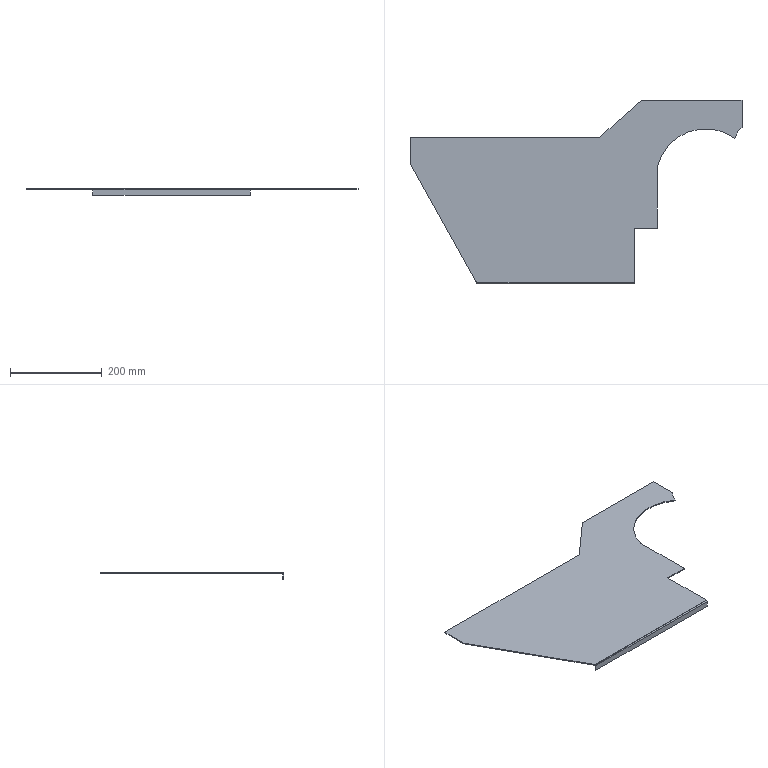Part | STEP file | TX-003-1 | 1 solid | 21 faces | box 722 x 399 x 15 mm | volume 342555 mm3 | plane 16 | cylinder 5 | commonest cylinder face diameters 1 x2 5 x1 78.426 x1 216 x1
STEP:
#1=CARTESIAN_POINT('',(-209.508,-144.397,0.));
#2=VERTEX_POINT('',#1);
#3=CARTESIAN_POINT('',(-209.508,-143.397,0.));
#4=VERTEX_POINT('',#3);
#5=CARTESIAN_POINT('',(-209.508,-143.397,0.));
#6=DIRECTION('',(0.,1.,0.));
#7=VECTOR('',#6,1000.);
#8=LINE('',#5,#7);
#9=EDGE_CURVE('',#2,#4,#8,.T.);
#10=ORIENTED_EDGE('',*,*,#9,.F.);
#11=CARTESIAN_POINT('',(132.378,-144.397,0.));
#12=VERTEX_POINT('',#11);
#13=CARTESIAN_POINT('',(287.878,-144.397,0.));
#14=DIRECTION('',(1.,0.,0.));
#15=VECTOR('',#14,1000.);
#16=LINE('',#13,#15);
#17=EDGE_CURVE('',#2,#12,#16,.T.);
#18=ORIENTED_EDGE('',*,*,#17,.T.);
#19=CARTESIAN_POINT('',(132.378,-25.897,0.));
#20=VERTEX_POINT('',#19);
#21=CARTESIAN_POINT('',(132.378,82.103,0.));
#22=DIRECTION('',(0.,1.,0.));
#23=VECTOR('',#22,1000.);
#24=LINE('',#21,#23);
#25=EDGE_CURVE('',#12,#20,#24,.T.);
#26=ORIENTED_EDGE('',*,*,#25,.T.);
#27=CARTESIAN_POINT('',(182.878,-25.897,0.));
#28=VERTEX_POINT('',#27);
#29=CARTESIAN_POINT('',(287.878,-25.897,0.));
#30=DIRECTION('',(1.,0.,0.));
#31=VECTOR('',#30,1000.);
#32=LINE('',#29,#31);
#33=EDGE_CURVE('',#20,#28,#32,.T.);
#34=ORIENTED_EDGE('',*,*,#33,.T.);
#35=CARTESIAN_POINT('',(182.878,107.381,0.));
#36=VERTEX_POINT('',#35);
#37=CARTESIAN_POINT('',(182.878,82.103,0.));
#38=DIRECTION('',(0.,1.,0.));
#39=VECTOR('',#38,1000.);
#40=LINE('',#37,#39);
#41=EDGE_CURVE('',#28,#36,#40,.T.);
#42=ORIENTED_EDGE('',*,*,#41,.T.);
#43=CARTESIAN_POINT('',(351.619,169.287,0.));
#44=VERTEX_POINT('',#43);
#45=CARTESIAN_POINT('',(287.878,82.103,0.));
#46=DIRECTION('',(0.,0.,-1.));
#47=DIRECTION('',(1.,0.,0.));
#48=AXIS2_PLACEMENT_3D('',#45,#46,#47);
#49=CIRCLE('',#48,108.);
#50=EDGE_CURVE('',#36,#44,#49,.T.);
#51=ORIENTED_EDGE('',*,*,#50,.T.);
#52=CARTESIAN_POINT('',(366.878,193.103,0.));
#53=VERTEX_POINT('',#52);
#54=CARTESIAN_POINT('',(390.044,161.464,0.));
#55=DIRECTION('',(0.,0.,-1.));
#56=DIRECTION('',(1.,0.,0.));
#57=AXIS2_PLACEMENT_3D('',#54,#55,#56);
#58=CIRCLE('',#57,39.213);
#59=EDGE_CURVE('',#44,#53,#58,.T.);
#60=ORIENTED_EDGE('',*,*,#59,.T.);
#61=CARTESIAN_POINT('',(366.878,252.103,0.));
#62=VERTEX_POINT('',#61);
#63=CARTESIAN_POINT('',(366.878,82.103,0.));
#64=DIRECTION('',(0.,1.,0.));
#65=VECTOR('',#64,1000.);
#66=LINE('',#63,#65);
#67=EDGE_CURVE('',#53,#62,#66,.T.);
#68=ORIENTED_EDGE('',*,*,#67,.T.);
#69=CARTESIAN_POINT('',(147.878,252.103,0.));
#70=VERTEX_POINT('',#69);
#71=CARTESIAN_POINT('',(287.878,252.103,0.));
#72=DIRECTION('',(-1.,0.,0.));
#73=VECTOR('',#72,1000.);
#74=LINE('',#71,#73);
#75=EDGE_CURVE('',#62,#70,#74,.T.);
#76=ORIENTED_EDGE('',*,*,#75,.T.);
#77=CARTESIAN_POINT('',(57.878,172.103,0.));
#78=VERTEX_POINT('',#77);
#79=CARTESIAN_POINT('',(147.878,252.103,0.));
#80=DIRECTION('',(-0.7474,-0.6644,0.));
#81=VECTOR('',#80,1000.);
#82=LINE('',#79,#81);
#83=EDGE_CURVE('',#70,#78,#82,.T.);
#84=ORIENTED_EDGE('',*,*,#83,.T.);
#85=CARTESIAN_POINT('',(-355.122,172.103,0.));
#86=VERTEX_POINT('',#85);
#87=CARTESIAN_POINT('',(287.878,172.103,0.));
#88=DIRECTION('',(-1.,0.,0.));
#89=VECTOR('',#88,1000.);
#90=LINE('',#87,#89);
#91=EDGE_CURVE('',#78,#86,#90,.T.);
#92=ORIENTED_EDGE('',*,*,#91,.T.);
#93=CARTESIAN_POINT('',(-355.122,114.103,0.));
#94=VERTEX_POINT('',#93);
#95=CARTESIAN_POINT('',(-355.122,82.103,0.));
#96=DIRECTION('',(0.,-1.,0.));
#97=VECTOR('',#96,1000.);
#98=LINE('',#95,#97);
#99=EDGE_CURVE('',#86,#94,#98,.T.);
#100=ORIENTED_EDGE('',*,*,#99,.T.);
#101=CARTESIAN_POINT('',(-210.508,-145.105,0.));
#102=VERTEX_POINT('',#101);
#103=CARTESIAN_POINT('',(-355.122,114.103,0.));
#104=DIRECTION('',(0.4872,-0.8733,0.));
#105=VECTOR('',#104,1000.);
#106=LINE('',#103,#105);
#107=EDGE_CURVE('',#94,#102,#106,.T.);
#108=ORIENTED_EDGE('',*,*,#107,.T.);
#109=CARTESIAN_POINT('',(-210.508,-143.397,0.));
#110=VERTEX_POINT('',#109);
#111=CARTESIAN_POINT('',(-210.508,-145.105,0.));
#112=DIRECTION('',(0.,-1.,0.));
#113=VECTOR('',#112,1000.);
#114=LINE('',#111,#113);
#115=EDGE_CURVE('',#110,#102,#114,.T.);
#116=ORIENTED_EDGE('',*,*,#115,.F.);
#117=CARTESIAN_POINT('',(-210.008,-143.397,0.));
#118=DIRECTION('',(0.,0.,-1.));
#119=DIRECTION('',(1.,0.,0.));
#120=AXIS2_PLACEMENT_3D('',#117,#118,#119);
#121=CIRCLE('',#120,0.5);
#122=EDGE_CURVE('',#110,#4,#121,.T.);
#123=ORIENTED_EDGE('',*,*,#122,.T.);
#124=EDGE_LOOP('',(#10,#18,#26,#34,#42,#51,#60,#68,#76,#84,#92,#100,#108,#116,#123));
#125=FACE_OUTER_BOUND('',#124,.T.);
#126=CARTESIAN_POINT('',(287.878,82.103,0.));
#127=DIRECTION('',(0.,0.,1.));
#128=DIRECTION('',(1.,0.,0.));
#129=AXIS2_PLACEMENT_3D('',#126,#127,#128);
#130=PLANE('',#129);
#131=ADVANCED_FACE('',(#125),#130,.T.);
#132=CARTESIAN_POINT('',(-209.508,-146.897,-2.5));
#133=VERTEX_POINT('',#132);
#134=CARTESIAN_POINT('',(-209.508,-144.397,-2.5));
#135=DIRECTION('',(1.,0.,0.));
#136=DIRECTION('',(0.,0.,1.));
#137=AXIS2_PLACEMENT_3D('',#134,#135,#136);
#138=CIRCLE('',#137,2.5);
#139=EDGE_CURVE('',#2,#133,#138,.T.);
#140=ORIENTED_EDGE('',*,*,#139,.T.);
#141=CARTESIAN_POINT('',(132.378,-146.897,-2.5));
#142=VERTEX_POINT('',#141);
#143=CARTESIAN_POINT('',(-209.508,-146.897,-2.5));
#144=DIRECTION('',(1.,0.,0.));
#145=VECTOR('',#144,1000.);
#146=LINE('',#143,#145);
#147=EDGE_CURVE('',#133,#142,#146,.T.);
#148=ORIENTED_EDGE('',*,*,#147,.T.);
#149=CARTESIAN_POINT('',(132.378,-144.397,-2.5));
#150=DIRECTION('',(-1.,0.,0.));
#151=DIRECTION('',(0.,0.,1.));
#152=AXIS2_PLACEMENT_3D('',#149,#150,#151);
#153=CIRCLE('',#152,2.5);
#154=EDGE_CURVE('',#142,#12,#153,.T.);
#155=ORIENTED_EDGE('',*,*,#154,.T.);
#156=ORIENTED_EDGE('',*,*,#17,.F.);
#157=EDGE_LOOP('',(#140,#148,#155,#156));
#158=FACE_OUTER_BOUND('',#157,.T.);
#159=CARTESIAN_POINT('',(-209.508,-144.397,-2.5));
#160=DIRECTION('',(-1.,0.,0.));
#161=DIRECTION('',(0.,0.,1.));
#162=AXIS2_PLACEMENT_3D('',#159,#160,#161);
#163=CYLINDRICAL_SURFACE('',#162,2.5);
#164=ADVANCED_FACE('',(#158),#163,.T.);
#165=ORIENTED_EDGE('',*,*,#107,.F.);
#166=CARTESIAN_POINT('',(-355.122,114.103,-2.));
#167=VERTEX_POINT('',#166);
#168=CARTESIAN_POINT('',(-355.122,114.103,-2.));
#169=DIRECTION('',(0.,0.,-1.));
#170=VECTOR('',#169,1000.);
#171=LINE('',#168,#170);
#172=EDGE_CURVE('',#94,#167,#171,.T.);
#173=ORIENTED_EDGE('',*,*,#172,.T.);
#174=CARTESIAN_POINT('',(-210.508,-145.105,-2.));
#175=VERTEX_POINT('',#174);
#176=CARTESIAN_POINT('',(-355.122,114.103,-2.));
#177=DIRECTION('',(0.4872,-0.8733,0.));
#178=VECTOR('',#177,1000.);
#179=LINE('',#176,#178);
#180=EDGE_CURVE('',#167,#175,#179,.T.);
#181=ORIENTED_EDGE('',*,*,#180,.T.);
#182=CARTESIAN_POINT('',(-210.508,-145.105,-2.));
#183=DIRECTION('',(0.,0.,1.));
#184=VECTOR('',#183,1000.);
#185=LINE('',#182,#184);
#186=EDGE_CURVE('',#175,#102,#185,.T.);
#187=ORIENTED_EDGE('',*,*,#186,.T.);
#188=EDGE_LOOP('',(#165,#173,#181,#187));
#189=FACE_OUTER_BOUND('',#188,.T.);
#190=CARTESIAN_POINT('',(-355.122,114.103,-2.));
#191=DIRECTION('',(-0.8733,-0.4872,0.));
#192=DIRECTION('',(0.4872,-0.8733,0.));
#193=AXIS2_PLACEMENT_3D('',#190,#191,#192);
#194=PLANE('',#193);
#195=ADVANCED_FACE('',(#189),#194,.T.);
#196=CARTESIAN_POINT('',(-355.122,172.103,-2.));
#197=VERTEX_POINT('',#196);
#198=CARTESIAN_POINT('',(-355.122,114.103,-2.));
#199=DIRECTION('',(0.,-1.,0.));
#200=VECTOR('',#199,1000.);
#201=LINE('',#198,#200);
#202=EDGE_CURVE('',#197,#167,#201,.T.);
#203=ORIENTED_EDGE('',*,*,#202,.T.);
#204=ORIENTED_EDGE('',*,*,#172,.F.);
#205=ORIENTED_EDGE('',*,*,#99,.F.);
#206=CARTESIAN_POINT('',(-355.122,172.103,-2.));
#207=DIRECTION('',(0.,0.,-1.));
#208=VECTOR('',#207,1000.);
#209=LINE('',#206,#208);
#210=EDGE_CURVE('',#86,#197,#209,.T.);
#211=ORIENTED_EDGE('',*,*,#210,.T.);
#212=EDGE_LOOP('',(#203,#204,#205,#211));
#213=FACE_OUTER_BOUND('',#212,.T.);
#214=CARTESIAN_POINT('',(-355.122,114.103,-2.));
#215=DIRECTION('',(-1.,0.,0.));
#216=DIRECTION('',(0.,-1.,0.));
#217=AXIS2_PLACEMENT_3D('',#214,#215,#216);
#218=PLANE('',#217);
#219=ADVANCED_FACE('',(#213),#218,.T.);
#220=CARTESIAN_POINT('',(57.878,172.103,-2.));
#221=VERTEX_POINT('',#220);
#222=CARTESIAN_POINT('',(-355.122,172.103,-2.));
#223=DIRECTION('',(-1.,0.,0.));
#224=VECTOR('',#223,1000.);
#225=LINE('',#222,#224);
#226=EDGE_CURVE('',#221,#197,#225,.T.);
#227=ORIENTED_EDGE('',*,*,#226,.T.);
#228=ORIENTED_EDGE('',*,*,#210,.F.);
#229=ORIENTED_EDGE('',*,*,#91,.F.);
#230=CARTESIAN_POINT('',(57.878,172.103,-2.));
#231=DIRECTION('',(0.,0.,-1.));
#232=VECTOR('',#231,1000.);
#233=LINE('',#230,#232);
#234=EDGE_CURVE('',#78,#221,#233,.T.);
#235=ORIENTED_EDGE('',*,*,#234,.T.);
#236=EDGE_LOOP('',(#227,#228,#229,#235));
#237=FACE_OUTER_BOUND('',#236,.T.);
#238=CARTESIAN_POINT('',(-355.122,172.103,-2.));
#239=DIRECTION('',(0.,1.,0.));
#240=DIRECTION('',(-1.,0.,0.));
#241=AXIS2_PLACEMENT_3D('',#238,#239,#240);
#242=PLANE('',#241);
#243=ADVANCED_FACE('',(#237),#242,.T.);
#244=CARTESIAN_POINT('',(147.878,252.103,-2.));
#245=VERTEX_POINT('',#244);
#246=CARTESIAN_POINT('',(57.878,172.103,-2.));
#247=DIRECTION('',(-0.7474,-0.6644,0.));
#248=VECTOR('',#247,1000.);
#249=LINE('',#246,#248);
#250=EDGE_CURVE('',#245,#221,#249,.T.);
#251=ORIENTED_EDGE('',*,*,#250,.T.);
#252=ORIENTED_EDGE('',*,*,#234,.F.);
#253=ORIENTED_EDGE('',*,*,#83,.F.);
#254=CARTESIAN_POINT('',(147.878,252.103,-2.));
#255=DIRECTION('',(0.,0.,-1.));
#256=VECTOR('',#255,1000.);
#257=LINE('',#254,#256);
#258=EDGE_CURVE('',#70,#245,#257,.T.);
#259=ORIENTED_EDGE('',*,*,#258,.T.);
#260=EDGE_LOOP('',(#251,#252,#253,#259));
#261=FACE_OUTER_BOUND('',#260,.T.);
#262=CARTESIAN_POINT('',(57.878,172.103,-2.));
#263=DIRECTION('',(-0.6644,0.7474,0.));
#264=DIRECTION('',(-0.7474,-0.6644,0.));
#265=AXIS2_PLACEMENT_3D('',#262,#263,#264);
#266=PLANE('',#265);
#267=ADVANCED_FACE('',(#261),#266,.T.);
#268=CARTESIAN_POINT('',(366.878,252.103,-2.));
#269=VERTEX_POINT('',#268);
#270=CARTESIAN_POINT('',(147.878,252.103,-2.));
#271=DIRECTION('',(-1.,0.,0.));
#272=VECTOR('',#271,1000.);
#273=LINE('',#270,#272);
#274=EDGE_CURVE('',#269,#245,#273,.T.);
#275=ORIENTED_EDGE('',*,*,#274,.T.);
#276=ORIENTED_EDGE('',*,*,#258,.F.);
#277=ORIENTED_EDGE('',*,*,#75,.F.);
#278=CARTESIAN_POINT('',(366.878,252.103,-2.));
#279=DIRECTION('',(0.,0.,-1.));
#280=VECTOR('',#279,1000.);
#281=LINE('',#278,#280);
#282=EDGE_CURVE('',#62,#269,#281,.T.);
#283=ORIENTED_EDGE('',*,*,#282,.T.);
#284=EDGE_LOOP('',(#275,#276,#277,#283));
#285=FACE_OUTER_BOUND('',#284,.T.);
#286=CARTESIAN_POINT('',(147.878,252.103,-2.));
#287=DIRECTION('',(0.,1.,0.));
#288=DIRECTION('',(-1.,0.,0.));
#289=AXIS2_PLACEMENT_3D('',#286,#287,#288);
#290=PLANE('',#289);
#291=ADVANCED_FACE('',(#285),#290,.T.);
#292=CARTESIAN_POINT('',(366.878,193.103,-2.));
#293=VERTEX_POINT('',#292);
#294=CARTESIAN_POINT('',(366.878,193.103,-2.));
#295=DIRECTION('',(0.,1.,0.));
#296=VECTOR('',#295,1000.);
#297=LINE('',#294,#296);
#298=EDGE_CURVE('',#293,#269,#297,.T.);
#299=ORIENTED_EDGE('',*,*,#298,.T.);
#300=ORIENTED_EDGE('',*,*,#282,.F.);
#301=ORIENTED_EDGE('',*,*,#67,.F.);
#302=CARTESIAN_POINT('',(366.878,193.103,-2.));
#303=DIRECTION('',(0.,0.,-1.));
#304=VECTOR('',#303,1000.);
#305=LINE('',#302,#304);
#306=EDGE_CURVE('',#53,#293,#305,.T.);
#307=ORIENTED_EDGE('',*,*,#306,.T.);
#308=EDGE_LOOP('',(#299,#300,#301,#307));
#309=FACE_OUTER_BOUND('',#308,.T.);
#310=CARTESIAN_POINT('',(366.878,193.103,-2.));
#311=DIRECTION('',(1.,0.,0.));
#312=DIRECTION('',(0.,0.,-1.));
#313=AXIS2_PLACEMENT_3D('',#310,#311,#312);
#314=PLANE('',#313);
#315=ADVANCED_FACE('',(#309),#314,.T.);
#316=CARTESIAN_POINT('',(351.619,169.287,-2.));
#317=VERTEX_POINT('',#316);
#318=CARTESIAN_POINT('',(351.619,169.287,-2.));
#319=DIRECTION('',(0.,0.,1.));
#320=VECTOR('',#319,1000.);
#321=LINE('',#318,#320);
#322=EDGE_CURVE('',#317,#44,#321,.T.);
#323=ORIENTED_EDGE('',*,*,#322,.F.);
#324=CARTESIAN_POINT('',(390.044,161.464,-2.));
#325=DIRECTION('',(0.,0.,1.));
#326=DIRECTION('',(1.,0.,0.));
#327=AXIS2_PLACEMENT_3D('',#324,#325,#326);
#328=CIRCLE('',#327,39.213);
#329=EDGE_CURVE('',#293,#317,#328,.T.);
#330=ORIENTED_EDGE('',*,*,#329,.F.);
#331=ORIENTED_EDGE('',*,*,#306,.F.);
#332=ORIENTED_EDGE('',*,*,#59,.F.);
#333=EDGE_LOOP('',(#323,#330,#331,#332));
#334=FACE_OUTER_BOUND('',#333,.T.);
#335=CARTESIAN_POINT('',(390.044,161.464,-2.));
#336=DIRECTION('',(0.,0.,1.));
#337=DIRECTION('',(1.,0.,0.));
#338=AXIS2_PLACEMENT_3D('',#335,#336,#337);
#339=CYLINDRICAL_SURFACE('',#338,39.213);
#340=ADVANCED_FACE('',(#334),#339,.F.);
#341=CARTESIAN_POINT('',(182.878,107.381,-2.));
#342=VERTEX_POINT('',#341);
#343=CARTESIAN_POINT('',(182.878,107.381,-2.));
#344=DIRECTION('',(0.,0.,1.));
#345=VECTOR('',#344,1000.);
#346=LINE('',#343,#345);
#347=EDGE_CURVE('',#342,#36,#346,.T.);
#348=ORIENTED_EDGE('',*,*,#347,.F.);
#349=CARTESIAN_POINT('',(287.878,82.103,-2.));
#350=DIRECTION('',(0.,0.,1.));
#351=DIRECTION('',(1.,0.,0.));
#352=AXIS2_PLACEMENT_3D('',#349,#350,#351);
#353=CIRCLE('',#352,108.);
#354=EDGE_CURVE('',#317,#342,#353,.T.);
#355=ORIENTED_EDGE('',*,*,#354,.F.);
#356=ORIENTED_EDGE('',*,*,#322,.T.);
#357=ORIENTED_EDGE('',*,*,#50,.F.);
#358=EDGE_LOOP('',(#348,#355,#356,#357));
#359=FACE_OUTER_BOUND('',#358,.T.);
#360=CARTESIAN_POINT('',(287.878,82.103,-2.));
#361=DIRECTION('',(0.,0.,1.));
#362=DIRECTION('',(1.,0.,0.));
#363=AXIS2_PLACEMENT_3D('',#360,#361,#362);
#364=CYLINDRICAL_SURFACE('',#363,108.);
#365=ADVANCED_FACE('',(#359),#364,.F.);
#366=ORIENTED_EDGE('',*,*,#347,.T.);
#367=ORIENTED_EDGE('',*,*,#41,.F.);
#368=CARTESIAN_POINT('',(182.878,-25.897,-2.));
#369=VERTEX_POINT('',#368);
#370=CARTESIAN_POINT('',(182.878,-25.897,-2.));
#371=DIRECTION('',(0.,0.,-1.));
#372=VECTOR('',#371,1000.);
#373=LINE('',#370,#372);
#374=EDGE_CURVE('',#28,#369,#373,.T.);
#375=ORIENTED_EDGE('',*,*,#374,.T.);
#376=CARTESIAN_POINT('',(182.878,107.381,-2.));
#377=DIRECTION('',(0.,1.,0.));
#378=VECTOR('',#377,1000.);
#379=LINE('',#376,#378);
#380=EDGE_CURVE('',#369,#342,#379,.T.);
#381=ORIENTED_EDGE('',*,*,#380,.T.);
#382=EDGE_LOOP('',(#366,#367,#375,#381));
#383=FACE_OUTER_BOUND('',#382,.T.);
#384=CARTESIAN_POINT('',(182.878,107.381,-2.));
#385=DIRECTION('',(1.,0.,0.));
#386=DIRECTION('',(0.,1.,0.));
#387=AXIS2_PLACEMENT_3D('',#384,#385,#386);
#388=PLANE('',#387);
#389=ADVANCED_FACE('',(#383),#388,.T.);
#390=ORIENTED_EDGE('',*,*,#33,.F.);
#391=CARTESIAN_POINT('',(132.378,-25.897,-2.));
#392=VERTEX_POINT('',#391);
#393=CARTESIAN_POINT('',(132.378,-25.897,-15.));
#394=DIRECTION('',(0.,0.,1.));
#395=VECTOR('',#394,1000.);
#396=LINE('',#393,#395);
#397=EDGE_CURVE('',#392,#20,#396,.T.);
#398=ORIENTED_EDGE('',*,*,#397,.F.);
#399=CARTESIAN_POINT('',(182.878,-25.897,-2.));
#400=DIRECTION('',(-1.,0.,0.));
#401=VECTOR('',#400,1000.);
#402=LINE('',#399,#401);
#403=EDGE_CURVE('',#369,#392,#402,.T.);
#404=ORIENTED_EDGE('',*,*,#403,.F.);
#405=ORIENTED_EDGE('',*,*,#374,.F.);
#406=EDGE_LOOP('',(#390,#398,#404,#405));
#407=FACE_OUTER_BOUND('',#406,.T.);
#408=CARTESIAN_POINT('',(182.878,-25.897,-15.));
#409=DIRECTION('',(0.,1.,0.));
#410=DIRECTION('',(-1.,0.,0.));
#411=AXIS2_PLACEMENT_3D('',#408,#409,#410);
#412=PLANE('',#411);
#413=ADVANCED_FACE('',(#407),#412,.F.);
#414=CARTESIAN_POINT('',(132.378,-146.897,-15.));
#415=VERTEX_POINT('',#414);
#416=CARTESIAN_POINT('',(132.378,-146.897,-15.));
#417=DIRECTION('',(0.,0.,1.));
#418=VECTOR('',#417,1000.);
#419=LINE('',#416,#418);
#420=EDGE_CURVE('',#415,#142,#419,.T.);
#421=ORIENTED_EDGE('',*,*,#420,.F.);
#422=CARTESIAN_POINT('',(132.378,-144.897,-15.));
#423=VERTEX_POINT('',#422);
#424=CARTESIAN_POINT('',(132.378,-25.897,-15.));
#425=DIRECTION('',(0.,-1.,0.));
#426=VECTOR('',#425,1000.);
#427=LINE('',#424,#426);
#428=EDGE_CURVE('',#423,#415,#427,.T.);
#429=ORIENTED_EDGE('',*,*,#428,.F.);
#430=CARTESIAN_POINT('',(132.378,-144.897,-2.5));
#431=VERTEX_POINT('',#430);
#432=CARTESIAN_POINT('',(132.378,-144.897,-15.));
#433=DIRECTION('',(0.,0.,-1.));
#434=VECTOR('',#433,1000.);
#435=LINE('',#432,#434);
#436=EDGE_CURVE('',#431,#423,#435,.T.);
#437=ORIENTED_EDGE('',*,*,#436,.F.);
#438=CARTESIAN_POINT('',(132.378,-144.397,-2.));
#439=VERTEX_POINT('',#438);
#440=CARTESIAN_POINT('',(132.378,-144.397,-2.5));
#441=DIRECTION('',(-1.,0.,0.));
#442=DIRECTION('',(0.,0.,1.));
#443=AXIS2_PLACEMENT_3D('',#440,#441,#442);
#444=CIRCLE('',#443,0.5);
#445=EDGE_CURVE('',#431,#439,#444,.T.);
#446=ORIENTED_EDGE('',*,*,#445,.T.);
#447=CARTESIAN_POINT('',(132.378,-25.897,-2.));
#448=DIRECTION('',(0.,-1.,0.));
#449=VECTOR('',#448,1000.);
#450=LINE('',#447,#449);
#451=EDGE_CURVE('',#392,#439,#450,.T.);
#452=ORIENTED_EDGE('',*,*,#451,.F.);
#453=ORIENTED_EDGE('',*,*,#397,.T.);
#454=ORIENTED_EDGE('',*,*,#25,.F.);
#455=ORIENTED_EDGE('',*,*,#154,.F.);
#456=EDGE_LOOP('',(#421,#429,#437,#446,#452,#453,#454,#455));
#457=FACE_OUTER_BOUND('',#456,.T.);
#458=CARTESIAN_POINT('',(132.378,-25.897,-15.));
#459=DIRECTION('',(-1.,0.,0.));
#460=DIRECTION('',(0.,-1.,0.));
#461=AXIS2_PLACEMENT_3D('',#458,#459,#460);
#462=PLANE('',#461);
#463=ADVANCED_FACE('',(#457),#462,.F.);
#464=CARTESIAN_POINT('',(-209.508,-146.897,-15.));
#465=VERTEX_POINT('',#464);
#466=CARTESIAN_POINT('',(-209.508,-146.897,0.));
#467=DIRECTION('',(0.,0.,-1.));
#468=VECTOR('',#467,1000.);
#469=LINE('',#466,#468);
#470=EDGE_CURVE('',#133,#465,#469,.T.);
#471=ORIENTED_EDGE('',*,*,#470,.T.);
#472=CARTESIAN_POINT('',(0.,-146.897,-15.));
#473=DIRECTION('',(1.,0.,0.));
#474=VECTOR('',#473,1000.);
#475=LINE('',#472,#474);
#476=EDGE_CURVE('',#465,#415,#475,.T.);
#477=ORIENTED_EDGE('',*,*,#476,.T.);
#478=ORIENTED_EDGE('',*,*,#420,.T.);
#479=ORIENTED_EDGE('',*,*,#147,.F.);
#480=EDGE_LOOP('',(#471,#477,#478,#479));
#481=FACE_OUTER_BOUND('',#480,.T.);
#482=CARTESIAN_POINT('',(0.,-146.897,0.));
#483=DIRECTION('',(0.,-1.,0.));
#484=DIRECTION('',(0.,0.,-1.));
#485=AXIS2_PLACEMENT_3D('',#482,#483,#484);
#486=PLANE('',#485);
#487=ADVANCED_FACE('',(#481),#486,.T.);
#488=CARTESIAN_POINT('',(-209.508,-144.397,-2.));
#489=VERTEX_POINT('',#488);
#490=CARTESIAN_POINT('',(-209.508,-144.897,-2.5));
#491=VERTEX_POINT('',#490);
#492=CARTESIAN_POINT('',(-209.508,-144.397,-2.5));
#493=DIRECTION('',(1.,0.,0.));
#494=DIRECTION('',(0.,0.,1.));
#495=AXIS2_PLACEMENT_3D('',#492,#493,#494);
#496=CIRCLE('',#495,0.5);
#497=EDGE_CURVE('',#489,#491,#496,.T.);
#498=ORIENTED_EDGE('',*,*,#497,.T.);
#499=CARTESIAN_POINT('',(-209.508,-144.897,-15.));
#500=VERTEX_POINT('',#499);
#501=CARTESIAN_POINT('',(-209.508,-144.897,0.));
#502=DIRECTION('',(0.,0.,-1.));
#503=VECTOR('',#502,1000.);
#504=LINE('',#501,#503);
#505=EDGE_CURVE('',#491,#500,#504,.T.);
#506=ORIENTED_EDGE('',*,*,#505,.T.);
#507=CARTESIAN_POINT('',(-209.508,-146.897,-15.));
#508=DIRECTION('',(0.,1.,0.));
#509=VECTOR('',#508,1000.);
#510=LINE('',#507,#509);
#511=EDGE_CURVE('',#465,#500,#510,.T.);
#512=ORIENTED_EDGE('',*,*,#511,.F.);
#513=ORIENTED_EDGE('',*,*,#470,.F.);
#514=ORIENTED_EDGE('',*,*,#139,.F.);
#515=ORIENTED_EDGE('',*,*,#9,.T.);
#516=CARTESIAN_POINT('',(-209.508,-143.397,-2.));
#517=VERTEX_POINT('',#516);
#518=CARTESIAN_POINT('',(-209.508,-143.397,-2.));
#519=DIRECTION('',(0.,0.,-1.));
#520=VECTOR('',#519,1000.);
#521=LINE('',#518,#520);
#522=EDGE_CURVE('',#4,#517,#521,.T.);
#523=ORIENTED_EDGE('',*,*,#522,.T.);
#524=CARTESIAN_POINT('',(-209.508,82.103,-2.));
#525=DIRECTION('',(0.,-1.,0.));
#526=VECTOR('',#525,1000.);
#527=LINE('',#524,#526);
#528=EDGE_CURVE('',#517,#489,#527,.T.);
#529=ORIENTED_EDGE('',*,*,#528,.T.);
#530=EDGE_LOOP('',(#498,#506,#512,#513,#514,#515,#523,#529));
#531=FACE_OUTER_BOUND('',#530,.T.);
#532=CARTESIAN_POINT('',(-209.508,-144.397,-2.5));
#533=DIRECTION('',(1.,0.,0.));
#534=DIRECTION('',(0.,0.,-1.));
#535=AXIS2_PLACEMENT_3D('',#532,#533,#534);
#536=PLANE('',#535);
#537=ADVANCED_FACE('',(#531),#536,.F.);
#538=CARTESIAN_POINT('',(-210.508,-143.397,-2.));
#539=VERTEX_POINT('',#538);
#540=CARTESIAN_POINT('',(-210.508,-145.105,-2.));
#541=DIRECTION('',(0.,1.,0.));
#542=VECTOR('',#541,1000.);
#543=LINE('',#540,#542);
#544=EDGE_CURVE('',#175,#539,#543,.T.);
#545=ORIENTED_EDGE('',*,*,#544,.T.);
#546=CARTESIAN_POINT('',(-210.508,-143.397,-2.));
#547=DIRECTION('',(0.,0.,1.));
#548=VECTOR('',#547,1000.);
#549=LINE('',#546,#548);
#550=EDGE_CURVE('',#539,#110,#549,.T.);
#551=ORIENTED_EDGE('',*,*,#550,.T.);
#552=ORIENTED_EDGE('',*,*,#115,.T.);
#553=ORIENTED_EDGE('',*,*,#186,.F.);
#554=EDGE_LOOP('',(#545,#551,#552,#553));
#555=FACE_OUTER_BOUND('',#554,.T.);
#556=CARTESIAN_POINT('',(-210.508,-145.105,-2.));
#557=DIRECTION('',(1.,0.,0.));
#558=DIRECTION('',(0.,0.,-1.));
#559=AXIS2_PLACEMENT_3D('',#556,#557,#558);
#560=PLANE('',#559);
#561=ADVANCED_FACE('',(#555),#560,.T.);
#562=ORIENTED_EDGE('',*,*,#451,.T.);
#563=CARTESIAN_POINT('',(287.878,-144.397,-2.));
#564=DIRECTION('',(1.,0.,0.));
#565=VECTOR('',#564,1000.);
#566=LINE('',#563,#565);
#567=EDGE_CURVE('',#489,#439,#566,.T.);
#568=ORIENTED_EDGE('',*,*,#567,.F.);
#569=ORIENTED_EDGE('',*,*,#528,.F.);
#570=CARTESIAN_POINT('',(-210.008,-143.397,-2.));
#571=DIRECTION('',(0.,0.,-1.));
#572=DIRECTION('',(1.,0.,0.));
#573=AXIS2_PLACEMENT_3D('',#570,#571,#572);
#574=CIRCLE('',#573,0.5);
#575=EDGE_CURVE('',#539,#517,#574,.T.);
#576=ORIENTED_EDGE('',*,*,#575,.F.);
#577=ORIENTED_EDGE('',*,*,#544,.F.);
#578=ORIENTED_EDGE('',*,*,#180,.F.);
#579=ORIENTED_EDGE('',*,*,#202,.F.);
#580=ORIENTED_EDGE('',*,*,#226,.F.);
#581=ORIENTED_EDGE('',*,*,#250,.F.);
#582=ORIENTED_EDGE('',*,*,#274,.F.);
#583=ORIENTED_EDGE('',*,*,#298,.F.);
#584=ORIENTED_EDGE('',*,*,#329,.T.);
#585=ORIENTED_EDGE('',*,*,#354,.T.);
#586=ORIENTED_EDGE('',*,*,#380,.F.);
#587=ORIENTED_EDGE('',*,*,#403,.T.);
#588=EDGE_LOOP('',(#562,#568,#569,#576,#577,#578,#579,#580,#581,#582,#583,#584,#585,#586,#587));
#589=FACE_OUTER_BOUND('',#588,.T.);
#590=CARTESIAN_POINT('',(287.878,82.103,-2.));
#591=DIRECTION('',(0.,0.,1.));
#592=DIRECTION('',(1.,0.,0.));
#593=AXIS2_PLACEMENT_3D('',#590,#591,#592);
#594=PLANE('',#593);
#595=ADVANCED_FACE('',(#589),#594,.F.);
#596=ORIENTED_EDGE('',*,*,#511,.T.);
#597=CARTESIAN_POINT('',(-209.508,-144.897,-15.));
#598=DIRECTION('',(1.,0.,0.));
#599=VECTOR('',#598,1000.);
#600=LINE('',#597,#599);
#601=EDGE_CURVE('',#500,#423,#600,.T.);
#602=ORIENTED_EDGE('',*,*,#601,.T.);
#603=ORIENTED_EDGE('',*,*,#428,.T.);
#604=ORIENTED_EDGE('',*,*,#476,.F.);
#605=EDGE_LOOP('',(#596,#602,#603,#604));
#606=FACE_OUTER_BOUND('',#605,.T.);
#607=CARTESIAN_POINT('',(-209.508,-146.897,-15.));
#608=DIRECTION('',(0.,0.,-1.));
#609=DIRECTION('',(0.,1.,0.));
#610=AXIS2_PLACEMENT_3D('',#607,#608,#609);
#611=PLANE('',#610);
#612=ADVANCED_FACE('',(#606),#611,.T.);
#613=ORIENTED_EDGE('',*,*,#436,.T.);
#614=ORIENTED_EDGE('',*,*,#601,.F.);
#615=ORIENTED_EDGE('',*,*,#505,.F.);
#616=CARTESIAN_POINT('',(0.,-144.897,-2.5));
#617=DIRECTION('',(-1.,0.,0.));
#618=VECTOR('',#617,1000.);
#619=LINE('',#616,#618);
#620=EDGE_CURVE('',#431,#491,#619,.T.);
#621=ORIENTED_EDGE('',*,*,#620,.F.);
#622=EDGE_LOOP('',(#613,#614,#615,#621));
#623=FACE_OUTER_BOUND('',#622,.T.);
#624=CARTESIAN_POINT('',(0.,-144.897,0.));
#625=DIRECTION('',(0.,-1.,0.));
#626=DIRECTION('',(0.,0.,-1.));
#627=AXIS2_PLACEMENT_3D('',#624,#625,#626);
#628=PLANE('',#627);
#629=ADVANCED_FACE('',(#623),#628,.F.);
#630=ORIENTED_EDGE('',*,*,#550,.F.);
#631=ORIENTED_EDGE('',*,*,#575,.T.);
#632=ORIENTED_EDGE('',*,*,#522,.F.);
#633=ORIENTED_EDGE('',*,*,#122,.F.);
#634=EDGE_LOOP('',(#630,#631,#632,#633));
#635=FACE_OUTER_BOUND('',#634,.T.);
#636=CARTESIAN_POINT('',(-210.008,-143.397,-2.));
#637=DIRECTION('',(0.,0.,1.));
#638=DIRECTION('',(1.,0.,0.));
#639=AXIS2_PLACEMENT_3D('',#636,#637,#638);
#640=CYLINDRICAL_SURFACE('',#639,0.5);
#641=ADVANCED_FACE('',(#635),#640,.F.);
#642=ORIENTED_EDGE('',*,*,#445,.F.);
#643=ORIENTED_EDGE('',*,*,#620,.T.);
#644=ORIENTED_EDGE('',*,*,#497,.F.);
#645=ORIENTED_EDGE('',*,*,#567,.T.);
#646=EDGE_LOOP('',(#642,#643,#644,#645));
#647=FACE_OUTER_BOUND('',#646,.T.);
#648=CARTESIAN_POINT('',(-209.508,-144.397,-2.5));
#649=DIRECTION('',(-1.,0.,0.));
#650=DIRECTION('',(0.,0.,1.));
#651=AXIS2_PLACEMENT_3D('',#648,#649,#650);
#652=CYLINDRICAL_SURFACE('',#651,0.5);
#653=ADVANCED_FACE('',(#647),#652,.F.);
#654=CLOSED_SHELL('',(#131,#164,#195,#219,#243,#267,#291,#315,#340,#365,#389,#413,#463,#487,#537,#561,#595,#612,#629,#641,#653));
#655=MANIFOLD_SOLID_BREP('',#654);
#656=CARTESIAN_POINT('',(0.,0.,0.));
#657=DIRECTION('',(0.,0.,1.));
#658=DIRECTION('',(1.,0.,0.));
#659=AXIS2_PLACEMENT_3D('',#656,#657,#658);
#660=(LENGTH_UNIT()NAMED_UNIT(*)SI_UNIT(.MILLI.,.METRE.));
#661=UNCERTAINTY_MEASURE_WITH_UNIT(LENGTH_MEASURE(0.00001),#660,'','');
#662=(NAMED_UNIT(*)PLANE_ANGLE_UNIT()SI_UNIT($,.RADIAN.));
#663=(NAMED_UNIT(*)SI_UNIT($,.STERADIAN.)SOLID_ANGLE_UNIT());
#664=(GEOMETRIC_REPRESENTATION_CONTEXT(3)GLOBAL_UNCERTAINTY_ASSIGNED_CONTEXT((#661))GLOBAL_UNIT_ASSIGNED_CONTEXT((#660,#662,#663))REPRESENTATION_CONTEXT('',''));
#665=ADVANCED_BREP_SHAPE_REPRESENTATION('',(#655,#659),#664);